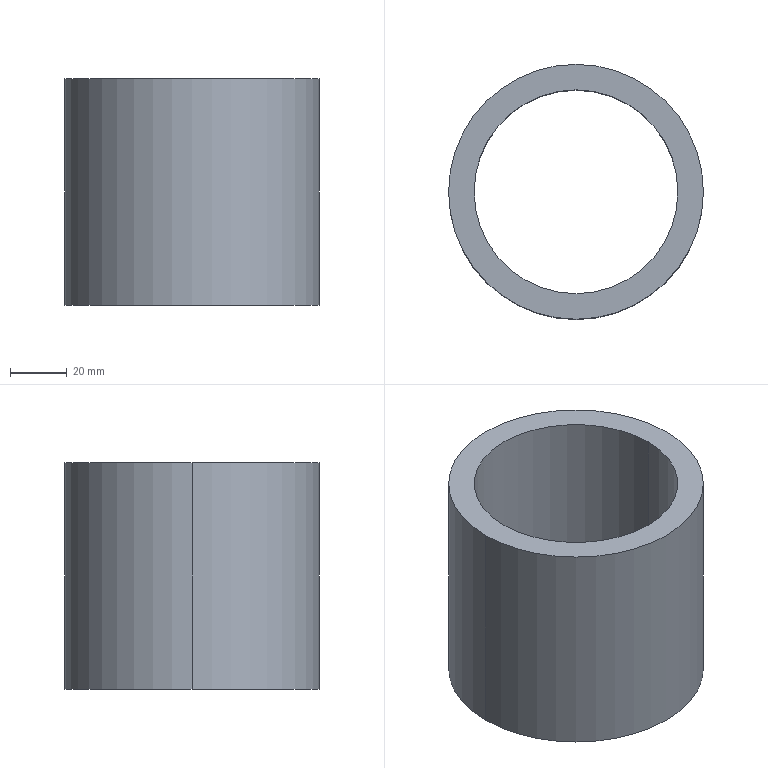Part | SolidWorks | features MirrorStock 1 | 1 solid | 6 faces | box 90 x 90 x 80 mm | volume 183218 mm3 | cylinder 4 | plane 2 | commonest cylinder face diameters 72 x2 90 x2
STEP:
#1=CARTESIAN_POINT('',(36.,0.,-40.));
#2=VERTEX_POINT('',#1);
#3=CARTESIAN_POINT('',(-36.,0.,-40.));
#4=VERTEX_POINT('',#3);
#5=CARTESIAN_POINT('',(0.,0.,-40.));
#6=DIRECTION('',(0.,0.,1.));
#7=DIRECTION('',(1.,0.,0.));
#8=AXIS2_PLACEMENT_3D('',#5,#6,#7);
#9=CIRCLE('',#8,36.);
#10=EDGE_CURVE('',#2,#4,#9,.T.);
#11=ORIENTED_EDGE('',*,*,#10,.F.);
#12=CARTESIAN_POINT('',(36.,0.,40.));
#13=VERTEX_POINT('',#12);
#14=CARTESIAN_POINT('',(36.,0.,-40.));
#15=DIRECTION('',(0.,0.,1.));
#16=VECTOR('',#15,1000.);
#17=LINE('',#14,#16);
#18=EDGE_CURVE('',#2,#13,#17,.T.);
#19=ORIENTED_EDGE('',*,*,#18,.T.);
#20=CARTESIAN_POINT('',(-36.,0.,40.));
#21=VERTEX_POINT('',#20);
#22=CARTESIAN_POINT('',(0.,0.,40.));
#23=DIRECTION('',(0.,0.,1.));
#24=DIRECTION('',(1.,0.,0.));
#25=AXIS2_PLACEMENT_3D('',#22,#23,#24);
#26=CIRCLE('',#25,36.);
#27=EDGE_CURVE('',#13,#21,#26,.T.);
#28=ORIENTED_EDGE('',*,*,#27,.T.);
#29=CARTESIAN_POINT('',(-36.,0.,-40.));
#30=DIRECTION('',(0.,0.,1.));
#31=VECTOR('',#30,1000.);
#32=LINE('',#29,#31);
#33=EDGE_CURVE('',#4,#21,#32,.T.);
#34=ORIENTED_EDGE('',*,*,#33,.F.);
#35=EDGE_LOOP('',(#11,#19,#28,#34));
#36=FACE_OUTER_BOUND('',#35,.T.);
#37=CARTESIAN_POINT('',(0.,0.,-40.));
#38=DIRECTION('',(0.,0.,1.));
#39=DIRECTION('',(-1.,0.,0.));
#40=AXIS2_PLACEMENT_3D('',#37,#38,#39);
#41=CYLINDRICAL_SURFACE('',#40,36.);
#42=ADVANCED_FACE('',(#36),#41,.F.);
#43=CARTESIAN_POINT('',(-45.,0.,-40.));
#44=VERTEX_POINT('',#43);
#45=CARTESIAN_POINT('',(45.,0.,-40.));
#46=VERTEX_POINT('',#45);
#47=CARTESIAN_POINT('',(0.,0.,-40.));
#48=DIRECTION('',(0.,0.,1.));
#49=DIRECTION('',(1.,0.,0.));
#50=AXIS2_PLACEMENT_3D('',#47,#48,#49);
#51=CIRCLE('',#50,45.);
#52=EDGE_CURVE('',#44,#46,#51,.T.);
#53=ORIENTED_EDGE('',*,*,#52,.T.);
#54=CARTESIAN_POINT('',(45.,0.,40.));
#55=VERTEX_POINT('',#54);
#56=CARTESIAN_POINT('',(45.,0.,-40.));
#57=DIRECTION('',(0.,0.,1.));
#58=VECTOR('',#57,1000.);
#59=LINE('',#56,#58);
#60=EDGE_CURVE('',#46,#55,#59,.T.);
#61=ORIENTED_EDGE('',*,*,#60,.T.);
#62=CARTESIAN_POINT('',(-45.,0.,40.));
#63=VERTEX_POINT('',#62);
#64=CARTESIAN_POINT('',(0.,0.,40.));
#65=DIRECTION('',(0.,0.,1.));
#66=DIRECTION('',(1.,0.,0.));
#67=AXIS2_PLACEMENT_3D('',#64,#65,#66);
#68=CIRCLE('',#67,45.);
#69=EDGE_CURVE('',#63,#55,#68,.T.);
#70=ORIENTED_EDGE('',*,*,#69,.F.);
#71=CARTESIAN_POINT('',(-45.,0.,-40.));
#72=DIRECTION('',(0.,0.,1.));
#73=VECTOR('',#72,1000.);
#74=LINE('',#71,#73);
#75=EDGE_CURVE('',#44,#63,#74,.T.);
#76=ORIENTED_EDGE('',*,*,#75,.F.);
#77=EDGE_LOOP('',(#53,#61,#70,#76));
#78=FACE_OUTER_BOUND('',#77,.T.);
#79=CARTESIAN_POINT('',(0.,0.,-40.));
#80=DIRECTION('',(0.,0.,1.));
#81=DIRECTION('',(-1.,0.,0.));
#82=AXIS2_PLACEMENT_3D('',#79,#80,#81);
#83=CYLINDRICAL_SURFACE('',#82,45.);
#84=ADVANCED_FACE('',(#78),#83,.T.);
#85=ORIENTED_EDGE('',*,*,#52,.F.);
#86=CARTESIAN_POINT('',(0.,0.,-40.));
#87=DIRECTION('',(0.,0.,1.));
#88=DIRECTION('',(1.,0.,0.));
#89=AXIS2_PLACEMENT_3D('',#86,#87,#88);
#90=CIRCLE('',#89,45.);
#91=EDGE_CURVE('',#46,#44,#90,.T.);
#92=ORIENTED_EDGE('',*,*,#91,.F.);
#93=EDGE_LOOP('',(#85,#92));
#94=FACE_OUTER_BOUND('',#93,.T.);
#95=CARTESIAN_POINT('',(0.,0.,-40.));
#96=DIRECTION('',(0.,0.,1.));
#97=DIRECTION('',(1.,0.,0.));
#98=AXIS2_PLACEMENT_3D('',#95,#96,#97);
#99=CIRCLE('',#98,36.);
#100=EDGE_CURVE('',#4,#2,#99,.T.);
#101=ORIENTED_EDGE('',*,*,#100,.T.);
#102=ORIENTED_EDGE('',*,*,#10,.T.);
#103=EDGE_LOOP('',(#101,#102));
#104=FACE_BOUND('',#103,.T.);
#105=CARTESIAN_POINT('',(0.,0.,-40.));
#106=DIRECTION('',(0.,0.,-1.));
#107=DIRECTION('',(1.,0.,0.));
#108=AXIS2_PLACEMENT_3D('',#105,#106,#107);
#109=PLANE('',#108);
#110=ADVANCED_FACE('',(#94,#104),#109,.T.);
#111=ORIENTED_EDGE('',*,*,#69,.T.);
#112=CARTESIAN_POINT('',(0.,0.,40.));
#113=DIRECTION('',(0.,0.,1.));
#114=DIRECTION('',(1.,0.,0.));
#115=AXIS2_PLACEMENT_3D('',#112,#113,#114);
#116=CIRCLE('',#115,45.);
#117=EDGE_CURVE('',#55,#63,#116,.T.);
#118=ORIENTED_EDGE('',*,*,#117,.T.);
#119=EDGE_LOOP('',(#111,#118));
#120=FACE_OUTER_BOUND('',#119,.T.);
#121=CARTESIAN_POINT('',(0.,0.,40.));
#122=DIRECTION('',(0.,0.,1.));
#123=DIRECTION('',(1.,0.,0.));
#124=AXIS2_PLACEMENT_3D('',#121,#122,#123);
#125=CIRCLE('',#124,36.);
#126=EDGE_CURVE('',#21,#13,#125,.T.);
#127=ORIENTED_EDGE('',*,*,#126,.F.);
#128=ORIENTED_EDGE('',*,*,#27,.F.);
#129=EDGE_LOOP('',(#127,#128));
#130=FACE_BOUND('',#129,.T.);
#131=CARTESIAN_POINT('',(0.,0.,40.));
#132=DIRECTION('',(0.,0.,-1.));
#133=DIRECTION('',(1.,0.,0.));
#134=AXIS2_PLACEMENT_3D('',#131,#132,#133);
#135=PLANE('',#134);
#136=ADVANCED_FACE('',(#120,#130),#135,.F.);
#137=ORIENTED_EDGE('',*,*,#60,.F.);
#138=ORIENTED_EDGE('',*,*,#91,.T.);
#139=ORIENTED_EDGE('',*,*,#75,.T.);
#140=ORIENTED_EDGE('',*,*,#117,.F.);
#141=EDGE_LOOP('',(#137,#138,#139,#140));
#142=FACE_OUTER_BOUND('',#141,.T.);
#143=CARTESIAN_POINT('',(0.,0.,-40.));
#144=DIRECTION('',(0.,0.,1.));
#145=DIRECTION('',(-1.,0.,0.));
#146=AXIS2_PLACEMENT_3D('',#143,#144,#145);
#147=CYLINDRICAL_SURFACE('',#146,45.);
#148=ADVANCED_FACE('',(#142),#147,.T.);
#149=ORIENTED_EDGE('',*,*,#18,.F.);
#150=ORIENTED_EDGE('',*,*,#100,.F.);
#151=ORIENTED_EDGE('',*,*,#33,.T.);
#152=ORIENTED_EDGE('',*,*,#126,.T.);
#153=EDGE_LOOP('',(#149,#150,#151,#152));
#154=FACE_OUTER_BOUND('',#153,.T.);
#155=CARTESIAN_POINT('',(0.,0.,-40.));
#156=DIRECTION('',(0.,0.,1.));
#157=DIRECTION('',(-1.,0.,0.));
#158=AXIS2_PLACEMENT_3D('',#155,#156,#157);
#159=CYLINDRICAL_SURFACE('',#158,36.);
#160=ADVANCED_FACE('',(#154),#159,.F.);
#161=CLOSED_SHELL('',(#42,#84,#110,#136,#148,#160));
#162=MANIFOLD_SOLID_BREP('',#161);
#163=CARTESIAN_POINT('',(0.,0.,0.));
#164=DIRECTION('',(0.,0.,1.));
#165=DIRECTION('',(1.,0.,0.));
#166=AXIS2_PLACEMENT_3D('',#163,#164,#165);
#167=(LENGTH_UNIT()NAMED_UNIT(*)SI_UNIT(.MILLI.,.METRE.));
#168=UNCERTAINTY_MEASURE_WITH_UNIT(LENGTH_MEASURE(0.00001),#167,'','');
#169=(NAMED_UNIT(*)PLANE_ANGLE_UNIT()SI_UNIT($,.RADIAN.));
#170=(NAMED_UNIT(*)SI_UNIT($,.STERADIAN.)SOLID_ANGLE_UNIT());
#171=(GEOMETRIC_REPRESENTATION_CONTEXT(3)GLOBAL_UNCERTAINTY_ASSIGNED_CONTEXT((#168))GLOBAL_UNIT_ASSIGNED_CONTEXT((#167,#169,#170))REPRESENTATION_CONTEXT('',''));
#172=ADVANCED_BREP_SHAPE_REPRESENTATION('',(#162,#166),#171);